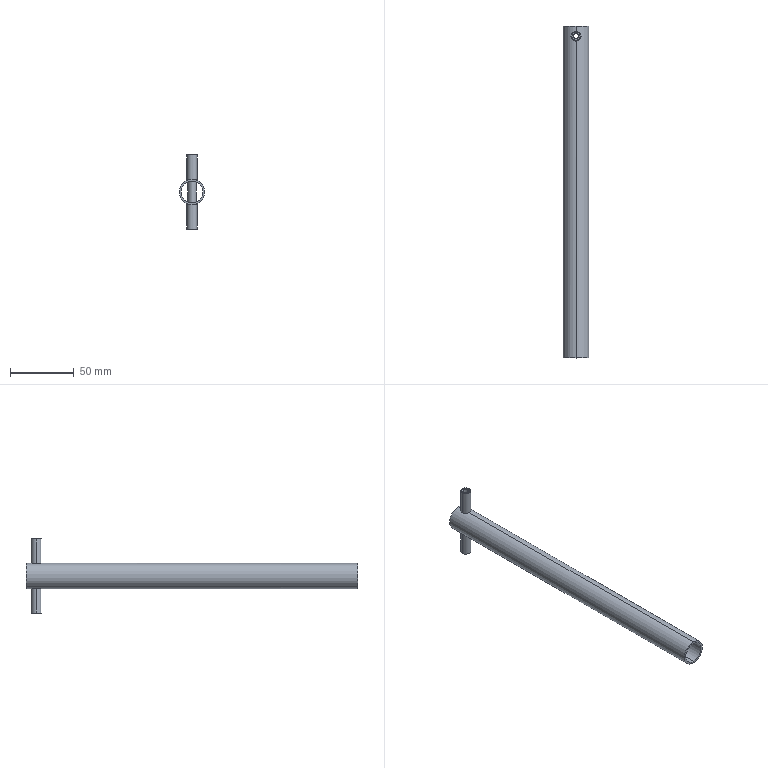Part | SolidWorks | features BaseBody 4 | 4 solids | 28 faces | box 20 x 260 x 58 mm | volume 24314 mm3 | cylinder 20 | plane 8 | commonest cylinder face diameters 6.3 x8 7.938 x4 4.166 x2 6.35 x2 17 x2 20 x2
STEP:
#1=CARTESIAN_POINT('',(0.,248.85,-10.));
#2=VERTEX_POINT('',#1);
#3=CARTESIAN_POINT('',(-3.15,252.,-9.491));
#4=VERTEX_POINT('',#3);
#5=CARTESIAN_POINT('',(0.,248.85,-10.));
#6=CARTESIAN_POINT('',(-0.2094,248.85,-10.));
#7=CARTESIAN_POINT('',(-0.4151,248.871,-9.993));
#8=CARTESIAN_POINT('',(-0.8193,248.951,-9.968));
#9=CARTESIAN_POINT('',(-1.02,249.013,-9.95));
#10=CARTESIAN_POINT('',(-1.401,249.171,-9.903));
#11=CARTESIAN_POINT('',(-1.581,249.268,-9.876));
#12=CARTESIAN_POINT('',(-1.922,249.496,-9.815));
#13=CARTESIAN_POINT('',(-2.083,249.628,-9.782));
#14=CARTESIAN_POINT('',(-2.516,250.061,-9.683));
#15=CARTESIAN_POINT('',(-2.75,250.41,-9.616));
#16=CARTESIAN_POINT('',(-2.986,250.977,-9.544));
#17=CARTESIAN_POINT('',(-3.047,251.176,-9.524));
#18=CARTESIAN_POINT('',(-3.129,251.584,-9.498));
#19=CARTESIAN_POINT('',(-3.15,251.791,-9.491));
#20=CARTESIAN_POINT('',(-3.15,252.,-9.491));
#21=B_SPLINE_CURVE_WITH_KNOTS('',3,(#5,#6,#7,#8,#9,#10,#11,#12,#13,#14,#15,#16,#17,#18,#19,#20),.UNSPECIFIED.,.F.,.F.,(4,2,2,2,2,2,2,4),(0.,0.0006191,0.001238,0.001857,0.002476,0.003715,0.004334,0.004953),.UNSPECIFIED.);
#22=EDGE_CURVE('',#2,#4,#21,.T.);
#23=ORIENTED_EDGE('',*,*,#22,.T.);
#24=CARTESIAN_POINT('',(-3.15,252.,-7.895));
#25=VERTEX_POINT('',#24);
#26=CARTESIAN_POINT('',(-3.15,252.,-10.013));
#27=DIRECTION('',(0.,0.,1.));
#28=VECTOR('',#27,1000.);
#29=LINE('',#26,#28);
#30=EDGE_CURVE('',#4,#25,#29,.T.);
#31=ORIENTED_EDGE('',*,*,#30,.T.);
#32=CARTESIAN_POINT('',(0.,248.85,-8.5));
#33=VERTEX_POINT('',#32);
#34=CARTESIAN_POINT('',(-3.15,252.,-7.895));
#35=CARTESIAN_POINT('',(-3.15,251.79,-7.895));
#36=CARTESIAN_POINT('',(-3.129,251.584,-7.903));
#37=CARTESIAN_POINT('',(-3.048,251.179,-7.935));
#38=CARTESIAN_POINT('',(-2.987,250.978,-7.958));
#39=CARTESIAN_POINT('',(-2.828,250.598,-8.016));
#40=CARTESIAN_POINT('',(-2.732,250.418,-8.05));
#41=CARTESIAN_POINT('',(-2.503,250.077,-8.124));
#42=CARTESIAN_POINT('',(-2.372,249.917,-8.164));
#43=CARTESIAN_POINT('',(-1.941,249.486,-8.281));
#44=CARTESIAN_POINT('',(-1.593,249.252,-8.358));
#45=CARTESIAN_POINT('',(-1.025,249.015,-8.44));
#46=CARTESIAN_POINT('',(-0.8254,248.953,-8.462));
#47=CARTESIAN_POINT('',(-0.4171,248.871,-8.492));
#48=CARTESIAN_POINT('',(-0.21,248.85,-8.5));
#49=CARTESIAN_POINT('',(0.,248.85,-8.5));
#50=B_SPLINE_CURVE_WITH_KNOTS('',3,(#34,#35,#36,#37,#38,#39,#40,#41,#42,#43,#44,#45,#46,#47,#48,#49),.UNSPECIFIED.,.F.,.F.,(4,2,2,2,2,2,2,4),(0.,0.0006207,0.001241,0.001862,0.002483,0.003724,0.004345,0.004966),.UNSPECIFIED.);
#51=EDGE_CURVE('',#25,#33,#50,.T.);
#52=ORIENTED_EDGE('',*,*,#51,.T.);
#53=CARTESIAN_POINT('',(3.15,252.,-7.895));
#54=VERTEX_POINT('',#53);
#55=CARTESIAN_POINT('',(0.,248.85,-8.5));
#56=CARTESIAN_POINT('',(0.21,248.85,-8.5));
#57=CARTESIAN_POINT('',(0.4162,248.871,-8.492));
#58=CARTESIAN_POINT('',(0.8212,248.952,-8.463));
#59=CARTESIAN_POINT('',(1.022,249.013,-8.441));
#60=CARTESIAN_POINT('',(1.403,249.172,-8.386));
#61=CARTESIAN_POINT('',(1.583,249.269,-8.353));
#62=CARTESIAN_POINT('',(1.924,249.497,-8.281));
#63=CARTESIAN_POINT('',(2.084,249.629,-8.242));
#64=CARTESIAN_POINT('',(2.515,250.06,-8.125));
#65=CARTESIAN_POINT('',(2.749,250.408,-8.045));
#66=CARTESIAN_POINT('',(2.986,250.975,-7.959));
#67=CARTESIAN_POINT('',(3.047,251.175,-7.935));
#68=CARTESIAN_POINT('',(3.129,251.583,-7.903));
#69=CARTESIAN_POINT('',(3.15,251.79,-7.895));
#70=CARTESIAN_POINT('',(3.15,252.,-7.895));
#71=B_SPLINE_CURVE_WITH_KNOTS('',3,(#55,#56,#57,#58,#59,#60,#61,#62,#63,#64,#65,#66,#67,#68,#69,#70),.UNSPECIFIED.,.F.,.F.,(4,2,2,2,2,2,2,4),(0.004966,0.005586,0.006207,0.006828,0.007448,0.00869,0.00931,0.009931),.UNSPECIFIED.);
#72=EDGE_CURVE('',#33,#54,#71,.T.);
#73=ORIENTED_EDGE('',*,*,#72,.T.);
#74=CARTESIAN_POINT('',(3.15,252.,-9.491));
#75=VERTEX_POINT('',#74);
#76=CARTESIAN_POINT('',(3.15,252.,-10.013));
#77=DIRECTION('',(0.,0.,1.));
#78=VECTOR('',#77,1000.);
#79=LINE('',#76,#78);
#80=EDGE_CURVE('',#75,#54,#79,.T.);
#81=ORIENTED_EDGE('',*,*,#80,.F.);
#82=CARTESIAN_POINT('',(3.15,252.,-9.491));
#83=CARTESIAN_POINT('',(3.15,251.791,-9.491));
#84=CARTESIAN_POINT('',(3.129,251.585,-9.498));
#85=CARTESIAN_POINT('',(3.049,251.181,-9.524));
#86=CARTESIAN_POINT('',(2.987,250.98,-9.544));
#87=CARTESIAN_POINT('',(2.829,250.6,-9.592));
#88=CARTESIAN_POINT('',(2.732,250.419,-9.62));
#89=CARTESIAN_POINT('',(2.504,250.078,-9.682));
#90=CARTESIAN_POINT('',(2.372,249.918,-9.716));
#91=CARTESIAN_POINT('',(1.94,249.485,-9.815));
#92=CARTESIAN_POINT('',(1.591,249.251,-9.88));
#93=CARTESIAN_POINT('',(1.024,249.014,-9.949));
#94=CARTESIAN_POINT('',(0.824,248.953,-9.968));
#95=CARTESIAN_POINT('',(0.4161,248.871,-9.993));
#96=CARTESIAN_POINT('',(0.2094,248.85,-10.));
#97=CARTESIAN_POINT('',(0.,248.85,-10.));
#98=B_SPLINE_CURVE_WITH_KNOTS('',3,(#82,#83,#84,#85,#86,#87,#88,#89,#90,#91,#92,#93,#94,#95,#96,#97),.UNSPECIFIED.,.F.,.F.,(4,2,2,2,2,2,2,4),(0.01486,0.01548,0.0161,0.01672,0.01733,0.01857,0.01919,0.01981),.UNSPECIFIED.);
#99=EDGE_CURVE('',#75,#2,#98,.T.);
#100=ORIENTED_EDGE('',*,*,#99,.T.);
#101=EDGE_LOOP('',(#23,#31,#52,#73,#81,#100));
#102=FACE_OUTER_BOUND('',#101,.T.);
#103=CARTESIAN_POINT('',(0.,252.,-10.013));
#104=DIRECTION('',(0.,0.,1.));
#105=DIRECTION('',(1.,0.,0.));
#106=AXIS2_PLACEMENT_3D('',#103,#104,#105);
#107=CYLINDRICAL_SURFACE('',#106,3.15);
#108=ADVANCED_FACE('',(#102),#107,.F.);
#109=CARTESIAN_POINT('',(0.,260.,10.));
#110=VERTEX_POINT('',#109);
#111=CARTESIAN_POINT('',(0.,260.,-10.));
#112=VERTEX_POINT('',#111);
#113=CARTESIAN_POINT('',(0.,260.,0.));
#114=DIRECTION('',(0.,1.,0.));
#115=DIRECTION('',(0.,0.,-1.));
#116=AXIS2_PLACEMENT_3D('',#113,#114,#115);
#117=CIRCLE('',#116,10.);
#118=EDGE_CURVE('',#110,#112,#117,.T.);
#119=ORIENTED_EDGE('',*,*,#118,.F.);
#120=CARTESIAN_POINT('',(0.,255.15,10.));
#121=VERTEX_POINT('',#120);
#122=CARTESIAN_POINT('',(0.,260.,10.));
#123=DIRECTION('',(0.,-1.,0.));
#124=VECTOR('',#123,1000.);
#125=LINE('',#122,#124);
#126=EDGE_CURVE('',#110,#121,#125,.T.);
#127=ORIENTED_EDGE('',*,*,#126,.T.);
#128=CARTESIAN_POINT('',(3.15,252.,9.491));
#129=VERTEX_POINT('',#128);
#130=CARTESIAN_POINT('',(3.15,252.,9.491));
#131=CARTESIAN_POINT('',(3.15,252.209,9.491));
#132=CARTESIAN_POINT('',(3.129,252.415,9.498));
#133=CARTESIAN_POINT('',(3.049,252.819,9.524));
#134=CARTESIAN_POINT('',(2.987,253.02,9.544));
#135=CARTESIAN_POINT('',(2.829,253.4,9.592));
#136=CARTESIAN_POINT('',(2.732,253.581,9.62));
#137=CARTESIAN_POINT('',(2.504,253.922,9.682));
#138=CARTESIAN_POINT('',(2.372,254.082,9.716));
#139=CARTESIAN_POINT('',(1.94,254.515,9.815));
#140=CARTESIAN_POINT('',(1.591,254.749,9.88));
#141=CARTESIAN_POINT('',(1.024,254.986,9.949));
#142=CARTESIAN_POINT('',(0.824,255.047,9.968));
#143=CARTESIAN_POINT('',(0.4161,255.129,9.993));
#144=CARTESIAN_POINT('',(0.2094,255.15,10.));
#145=CARTESIAN_POINT('',(0.,255.15,10.));
#146=B_SPLINE_CURVE_WITH_KNOTS('',3,(#130,#131,#132,#133,#134,#135,#136,#137,#138,#139,#140,#141,#142,#143,#144,#145),.UNSPECIFIED.,.F.,.F.,(4,2,2,2,2,2,2,4),(0.,0.0006191,0.001238,0.001857,0.002476,0.003714,0.004333,0.004953),.UNSPECIFIED.);
#147=EDGE_CURVE('',#129,#121,#146,.T.);
#148=ORIENTED_EDGE('',*,*,#147,.F.);
#149=CARTESIAN_POINT('',(0.,248.85,10.));
#150=VERTEX_POINT('',#149);
#151=CARTESIAN_POINT('',(0.,248.85,10.));
#152=CARTESIAN_POINT('',(0.2094,248.85,10.));
#153=CARTESIAN_POINT('',(0.4151,248.871,9.993));
#154=CARTESIAN_POINT('',(0.8193,248.951,9.968));
#155=CARTESIAN_POINT('',(1.02,249.013,9.95));
#156=CARTESIAN_POINT('',(1.401,249.171,9.903));
#157=CARTESIAN_POINT('',(1.581,249.268,9.876));
#158=CARTESIAN_POINT('',(1.922,249.496,9.815));
#159=CARTESIAN_POINT('',(2.083,249.628,9.782));
#160=CARTESIAN_POINT('',(2.516,250.061,9.683));
#161=CARTESIAN_POINT('',(2.75,250.41,9.616));
#162=CARTESIAN_POINT('',(2.986,250.977,9.544));
#163=CARTESIAN_POINT('',(3.047,251.176,9.524));
#164=CARTESIAN_POINT('',(3.129,251.584,9.498));
#165=CARTESIAN_POINT('',(3.15,251.791,9.491));
#166=CARTESIAN_POINT('',(3.15,252.,9.491));
#167=B_SPLINE_CURVE_WITH_KNOTS('',3,(#151,#152,#153,#154,#155,#156,#157,#158,#159,#160,#161,#162,#163,#164,#165,#166),.UNSPECIFIED.,.F.,.F.,(4,2,2,2,2,2,2,4),(-0.004952,-0.004333,-0.003714,-0.003095,-0.002476,-0.001238,-0.0006191,0.),.UNSPECIFIED.);
#168=EDGE_CURVE('',#150,#129,#167,.T.);
#169=ORIENTED_EDGE('',*,*,#168,.F.);
#170=CARTESIAN_POINT('',(0.,0.,10.));
#171=VERTEX_POINT('',#170);
#172=CARTESIAN_POINT('',(0.,260.,10.));
#173=DIRECTION('',(0.,-1.,0.));
#174=VECTOR('',#173,1000.);
#175=LINE('',#172,#174);
#176=EDGE_CURVE('',#150,#171,#175,.T.);
#177=ORIENTED_EDGE('',*,*,#176,.T.);
#178=CARTESIAN_POINT('',(0.,0.,-10.));
#179=VERTEX_POINT('',#178);
#180=CARTESIAN_POINT('',(0.,0.,0.));
#181=DIRECTION('',(0.,-1.,0.));
#182=DIRECTION('',(0.,0.,-1.));
#183=AXIS2_PLACEMENT_3D('',#180,#181,#182);
#184=CIRCLE('',#183,10.);
#185=EDGE_CURVE('',#179,#171,#184,.T.);
#186=ORIENTED_EDGE('',*,*,#185,.F.);
#187=CARTESIAN_POINT('',(0.,260.,-10.));
#188=DIRECTION('',(0.,-1.,0.));
#189=VECTOR('',#188,1000.);
#190=LINE('',#187,#189);
#191=EDGE_CURVE('',#2,#179,#190,.T.);
#192=ORIENTED_EDGE('',*,*,#191,.F.);
#193=ORIENTED_EDGE('',*,*,#99,.F.);
#194=CARTESIAN_POINT('',(0.,255.15,-10.));
#195=VERTEX_POINT('',#194);
#196=CARTESIAN_POINT('',(0.,255.15,-10.));
#197=CARTESIAN_POINT('',(0.2094,255.15,-10.));
#198=CARTESIAN_POINT('',(0.4151,255.129,-9.993));
#199=CARTESIAN_POINT('',(0.8193,255.049,-9.968));
#200=CARTESIAN_POINT('',(1.02,254.987,-9.95));
#201=CARTESIAN_POINT('',(1.401,254.829,-9.903));
#202=CARTESIAN_POINT('',(1.581,254.732,-9.876));
#203=CARTESIAN_POINT('',(1.922,254.504,-9.815));
#204=CARTESIAN_POINT('',(2.083,254.372,-9.782));
#205=CARTESIAN_POINT('',(2.516,253.939,-9.683));
#206=CARTESIAN_POINT('',(2.75,253.59,-9.616));
#207=CARTESIAN_POINT('',(2.986,253.023,-9.544));
#208=CARTESIAN_POINT('',(3.047,252.824,-9.524));
#209=CARTESIAN_POINT('',(3.129,252.416,-9.498));
#210=CARTESIAN_POINT('',(3.15,252.209,-9.491));
#211=CARTESIAN_POINT('',(3.15,252.,-9.491));
#212=B_SPLINE_CURVE_WITH_KNOTS('',3,(#196,#197,#198,#199,#200,#201,#202,#203,#204,#205,#206,#207,#208,#209,#210,#211),.UNSPECIFIED.,.F.,.F.,(4,2,2,2,2,2,2,4),(0.009906,0.01052,0.01114,0.01176,0.01238,0.01362,0.01424,0.01486),.UNSPECIFIED.);
#213=EDGE_CURVE('',#195,#75,#212,.T.);
#214=ORIENTED_EDGE('',*,*,#213,.F.);
#215=CARTESIAN_POINT('',(0.,260.,-10.));
#216=DIRECTION('',(0.,-1.,0.));
#217=VECTOR('',#216,1000.);
#218=LINE('',#215,#217);
#219=EDGE_CURVE('',#112,#195,#218,.T.);
#220=ORIENTED_EDGE('',*,*,#219,.F.);
#221=EDGE_LOOP('',(#119,#127,#148,#169,#177,#186,#192,#193,#214,#220));
#222=FACE_OUTER_BOUND('',#221,.T.);
#223=CARTESIAN_POINT('',(0.,260.,0.));
#224=DIRECTION('',(0.,-1.,0.));
#225=DIRECTION('',(0.,0.,-1.));
#226=AXIS2_PLACEMENT_3D('',#223,#224,#225);
#227=CYLINDRICAL_SURFACE('',#226,10.);
#228=ADVANCED_FACE('',(#222),#227,.T.);
#229=CARTESIAN_POINT('',(0.,260.,-8.5));
#230=VERTEX_POINT('',#229);
#231=CARTESIAN_POINT('',(0.,260.,8.5));
#232=VERTEX_POINT('',#231);
#233=CARTESIAN_POINT('',(0.,260.,0.));
#234=DIRECTION('',(0.,1.,0.));
#235=DIRECTION('',(0.,0.,-1.));
#236=AXIS2_PLACEMENT_3D('',#233,#234,#235);
#237=CIRCLE('',#236,8.5);
#238=EDGE_CURVE('',#230,#232,#237,.T.);
#239=ORIENTED_EDGE('',*,*,#238,.T.);
#240=CARTESIAN_POINT('',(0.,255.15,8.5));
#241=VERTEX_POINT('',#240);
#242=CARTESIAN_POINT('',(0.,260.,8.5));
#243=DIRECTION('',(0.,-1.,0.));
#244=VECTOR('',#243,1000.);
#245=LINE('',#242,#244);
#246=EDGE_CURVE('',#232,#241,#245,.T.);
#247=ORIENTED_EDGE('',*,*,#246,.T.);
#248=CARTESIAN_POINT('',(-3.15,252.,7.895));
#249=VERTEX_POINT('',#248);
#250=CARTESIAN_POINT('',(0.,255.15,8.5));
#251=CARTESIAN_POINT('',(-0.21,255.15,8.5));
#252=CARTESIAN_POINT('',(-0.4162,255.129,8.492));
#253=CARTESIAN_POINT('',(-0.8212,255.048,8.463));
#254=CARTESIAN_POINT('',(-1.022,254.987,8.441));
#255=CARTESIAN_POINT('',(-1.403,254.828,8.386));
#256=CARTESIAN_POINT('',(-1.583,254.731,8.353));
#257=CARTESIAN_POINT('',(-1.924,254.503,8.281));
#258=CARTESIAN_POINT('',(-2.084,254.371,8.242));
#259=CARTESIAN_POINT('',(-2.515,253.94,8.125));
#260=CARTESIAN_POINT('',(-2.749,253.592,8.045));
#261=CARTESIAN_POINT('',(-2.986,253.025,7.959));
#262=CARTESIAN_POINT('',(-3.047,252.825,7.935));
#263=CARTESIAN_POINT('',(-3.129,252.417,7.903));
#264=CARTESIAN_POINT('',(-3.15,252.21,7.895));
#265=CARTESIAN_POINT('',(-3.15,252.,7.895));
#266=B_SPLINE_CURVE_WITH_KNOTS('',3,(#250,#251,#252,#253,#254,#255,#256,#257,#258,#259,#260,#261,#262,#263,#264,#265),.UNSPECIFIED.,.F.,.F.,(4,2,2,2,2,2,2,4),(0.004966,0.005586,0.006207,0.006828,0.007448,0.00869,0.00931,0.009931),.UNSPECIFIED.);
#267=EDGE_CURVE('',#241,#249,#266,.T.);
#268=ORIENTED_EDGE('',*,*,#267,.T.);
#269=CARTESIAN_POINT('',(0.,248.85,8.5));
#270=VERTEX_POINT('',#269);
#271=CARTESIAN_POINT('',(-3.15,252.,7.895));
#272=CARTESIAN_POINT('',(-3.15,251.79,7.895));
#273=CARTESIAN_POINT('',(-3.129,251.584,7.903));
#274=CARTESIAN_POINT('',(-3.048,251.179,7.935));
#275=CARTESIAN_POINT('',(-2.987,250.978,7.958));
#276=CARTESIAN_POINT('',(-2.828,250.598,8.016));
#277=CARTESIAN_POINT('',(-2.732,250.418,8.05));
#278=CARTESIAN_POINT('',(-2.503,250.077,8.124));
#279=CARTESIAN_POINT('',(-2.372,249.917,8.164));
#280=CARTESIAN_POINT('',(-1.941,249.486,8.281));
#281=CARTESIAN_POINT('',(-1.593,249.252,8.358));
#282=CARTESIAN_POINT('',(-1.025,249.015,8.44));
#283=CARTESIAN_POINT('',(-0.8254,248.953,8.462));
#284=CARTESIAN_POINT('',(-0.4171,248.871,8.492));
#285=CARTESIAN_POINT('',(-0.21,248.85,8.5));
#286=CARTESIAN_POINT('',(0.,248.85,8.5));
#287=B_SPLINE_CURVE_WITH_KNOTS('',3,(#271,#272,#273,#274,#275,#276,#277,#278,#279,#280,#281,#282,#283,#284,#285,#286),.UNSPECIFIED.,.F.,.F.,(4,2,2,2,2,2,2,4),(-0.009931,-0.00931,-0.00869,-0.008069,-0.007448,-0.006207,-0.005586,-0.004966),.UNSPECIFIED.);
#288=EDGE_CURVE('',#249,#270,#287,.T.);
#289=ORIENTED_EDGE('',*,*,#288,.T.);
#290=CARTESIAN_POINT('',(0.,0.,8.5));
#291=VERTEX_POINT('',#290);
#292=CARTESIAN_POINT('',(0.,260.,8.5));
#293=DIRECTION('',(0.,-1.,0.));
#294=VECTOR('',#293,1000.);
#295=LINE('',#292,#294);
#296=EDGE_CURVE('',#270,#291,#295,.T.);
#297=ORIENTED_EDGE('',*,*,#296,.T.);
#298=CARTESIAN_POINT('',(0.,0.,-8.5));
#299=VERTEX_POINT('',#298);
#300=CARTESIAN_POINT('',(0.,0.,0.));
#301=DIRECTION('',(0.,-1.,0.));
#302=DIRECTION('',(0.,0.,-1.));
#303=AXIS2_PLACEMENT_3D('',#300,#301,#302);
#304=CIRCLE('',#303,8.5);
#305=EDGE_CURVE('',#291,#299,#304,.T.);
#306=ORIENTED_EDGE('',*,*,#305,.T.);
#307=CARTESIAN_POINT('',(0.,260.,-8.5));
#308=DIRECTION('',(0.,-1.,0.));
#309=VECTOR('',#308,1000.);
#310=LINE('',#307,#309);
#311=EDGE_CURVE('',#33,#299,#310,.T.);
#312=ORIENTED_EDGE('',*,*,#311,.F.);
#313=ORIENTED_EDGE('',*,*,#51,.F.);
#314=CARTESIAN_POINT('',(0.,255.15,-8.5));
#315=VERTEX_POINT('',#314);
#316=CARTESIAN_POINT('',(0.,255.15,-8.5));
#317=CARTESIAN_POINT('',(-0.21,255.15,-8.5));
#318=CARTESIAN_POINT('',(-0.4162,255.129,-8.492));
#319=CARTESIAN_POINT('',(-0.8212,255.048,-8.463));
#320=CARTESIAN_POINT('',(-1.022,254.987,-8.441));
#321=CARTESIAN_POINT('',(-1.403,254.828,-8.386));
#322=CARTESIAN_POINT('',(-1.583,254.731,-8.353));
#323=CARTESIAN_POINT('',(-1.924,254.503,-8.281));
#324=CARTESIAN_POINT('',(-2.084,254.371,-8.242));
#325=CARTESIAN_POINT('',(-2.515,253.94,-8.125));
#326=CARTESIAN_POINT('',(-2.749,253.592,-8.045));
#327=CARTESIAN_POINT('',(-2.986,253.025,-7.959));
#328=CARTESIAN_POINT('',(-3.047,252.825,-7.935));
#329=CARTESIAN_POINT('',(-3.129,252.417,-7.903));
#330=CARTESIAN_POINT('',(-3.15,252.21,-7.895));
#331=CARTESIAN_POINT('',(-3.15,252.,-7.895));
#332=B_SPLINE_CURVE_WITH_KNOTS('',3,(#316,#317,#318,#319,#320,#321,#322,#323,#324,#325,#326,#327,#328,#329,#330,#331),.UNSPECIFIED.,.F.,.F.,(4,2,2,2,2,2,2,4),(0.0149,0.01552,0.01614,0.01676,0.01738,0.01862,0.01924,0.01986),.UNSPECIFIED.);
#333=EDGE_CURVE('',#315,#25,#332,.T.);
#334=ORIENTED_EDGE('',*,*,#333,.F.);
#335=CARTESIAN_POINT('',(0.,260.,-8.5));
#336=DIRECTION('',(0.,-1.,0.));
#337=VECTOR('',#336,1000.);
#338=LINE('',#335,#337);
#339=EDGE_CURVE('',#230,#315,#338,.T.);
#340=ORIENTED_EDGE('',*,*,#339,.F.);
#341=EDGE_LOOP('',(#239,#247,#268,#289,#297,#306,#312,#313,#334,#340));
#342=FACE_OUTER_BOUND('',#341,.T.);
#343=CARTESIAN_POINT('',(0.,260.,0.));
#344=DIRECTION('',(0.,-1.,0.));
#345=DIRECTION('',(0.,0.,-1.));
#346=AXIS2_PLACEMENT_3D('',#343,#344,#345);
#347=CYLINDRICAL_SURFACE('',#346,8.5);
#348=ADVANCED_FACE('',(#342),#347,.F.);
#349=ORIENTED_EDGE('',*,*,#288,.F.);
#350=CARTESIAN_POINT('',(-3.15,252.,9.491));
#351=VERTEX_POINT('',#350);
#352=CARTESIAN_POINT('',(-3.15,252.,7.882));
#353=DIRECTION('',(0.,0.,1.));
#354=VECTOR('',#353,1000.);
#355=LINE('',#352,#354);
#356=EDGE_CURVE('',#249,#351,#355,.T.);
#357=ORIENTED_EDGE('',*,*,#356,.T.);
#358=CARTESIAN_POINT('',(-3.15,252.,9.491));
#359=CARTESIAN_POINT('',(-3.15,251.791,9.491));
#360=CARTESIAN_POINT('',(-3.129,251.585,9.498));
#361=CARTESIAN_POINT('',(-3.049,251.181,9.524));
#362=CARTESIAN_POINT('',(-2.987,250.98,9.544));
#363=CARTESIAN_POINT('',(-2.829,250.6,9.592));
#364=CARTESIAN_POINT('',(-2.732,250.419,9.62));
#365=CARTESIAN_POINT('',(-2.504,250.078,9.682));
#366=CARTESIAN_POINT('',(-2.372,249.918,9.716));
#367=CARTESIAN_POINT('',(-1.94,249.485,9.815));
#368=CARTESIAN_POINT('',(-1.591,249.251,9.88));
#369=CARTESIAN_POINT('',(-1.024,249.014,9.949));
#370=CARTESIAN_POINT('',(-0.824,248.953,9.968));
#371=CARTESIAN_POINT('',(-0.4161,248.871,9.993));
#372=CARTESIAN_POINT('',(-0.2094,248.85,10.));
#373=CARTESIAN_POINT('',(0.,248.85,10.));
#374=B_SPLINE_CURVE_WITH_KNOTS('',3,(#358,#359,#360,#361,#362,#363,#364,#365,#366,#367,#368,#369,#370,#371,#372,#373),.UNSPECIFIED.,.F.,.F.,(4,2,2,2,2,2,2,4),(0.009905,0.01052,0.01114,0.01176,0.01238,0.01362,0.01424,0.01486),.UNSPECIFIED.);
#375=EDGE_CURVE('',#351,#150,#374,.T.);
#376=ORIENTED_EDGE('',*,*,#375,.T.);
#377=ORIENTED_EDGE('',*,*,#168,.T.);
#378=CARTESIAN_POINT('',(3.15,252.,7.895));
#379=VERTEX_POINT('',#378);
#380=CARTESIAN_POINT('',(3.15,252.,7.882));
#381=DIRECTION('',(0.,0.,1.));
#382=VECTOR('',#381,1000.);
#383=LINE('',#380,#382);
#384=EDGE_CURVE('',#379,#129,#383,.T.);
#385=ORIENTED_EDGE('',*,*,#384,.F.);
#386=CARTESIAN_POINT('',(0.,248.85,8.5));
#387=CARTESIAN_POINT('',(0.21,248.85,8.5));
#388=CARTESIAN_POINT('',(0.4162,248.871,8.492));
#389=CARTESIAN_POINT('',(0.8212,248.952,8.463));
#390=CARTESIAN_POINT('',(1.022,249.013,8.441));
#391=CARTESIAN_POINT('',(1.403,249.172,8.386));
#392=CARTESIAN_POINT('',(1.583,249.269,8.353));
#393=CARTESIAN_POINT('',(1.924,249.497,8.281));
#394=CARTESIAN_POINT('',(2.084,249.629,8.242));
#395=CARTESIAN_POINT('',(2.515,250.06,8.125));
#396=CARTESIAN_POINT('',(2.749,250.408,8.045));
#397=CARTESIAN_POINT('',(2.986,250.975,7.959));
#398=CARTESIAN_POINT('',(3.047,251.175,7.935));
#399=CARTESIAN_POINT('',(3.129,251.583,7.903));
#400=CARTESIAN_POINT('',(3.15,251.79,7.895));
#401=CARTESIAN_POINT('',(3.15,252.,7.895));
#402=B_SPLINE_CURVE_WITH_KNOTS('',3,(#386,#387,#388,#389,#390,#391,#392,#393,#394,#395,#396,#397,#398,#399,#400,#401),.UNSPECIFIED.,.F.,.F.,(4,2,2,2,2,2,2,4),(-0.004966,-0.004345,-0.003724,-0.003103,-0.002483,-0.001241,-0.0006207,0.),.UNSPECIFIED.);
#403=EDGE_CURVE('',#270,#379,#402,.T.);
#404=ORIENTED_EDGE('',*,*,#403,.F.);
#405=EDGE_LOOP('',(#349,#357,#376,#377,#385,#404));
#406=FACE_OUTER_BOUND('',#405,.T.);
#407=CARTESIAN_POINT('',(0.,252.,7.882));
#408=DIRECTION('',(0.,0.,1.));
#409=DIRECTION('',(1.,0.,0.));
#410=AXIS2_PLACEMENT_3D('',#407,#408,#409);
#411=CYLINDRICAL_SURFACE('',#410,3.15);
#412=ADVANCED_FACE('',(#406),#411,.F.);
#413=ORIENTED_EDGE('',*,*,#30,.F.);
#414=CARTESIAN_POINT('',(-3.15,252.,-9.491));
#415=CARTESIAN_POINT('',(-3.15,252.209,-9.491));
#416=CARTESIAN_POINT('',(-3.129,252.415,-9.498));
#417=CARTESIAN_POINT('',(-3.049,252.819,-9.524));
#418=CARTESIAN_POINT('',(-2.987,253.02,-9.544));
#419=CARTESIAN_POINT('',(-2.829,253.4,-9.592));
#420=CARTESIAN_POINT('',(-2.732,253.581,-9.62));
#421=CARTESIAN_POINT('',(-2.504,253.922,-9.682));
#422=CARTESIAN_POINT('',(-2.372,254.082,-9.716));
#423=CARTESIAN_POINT('',(-1.94,254.515,-9.815));
#424=CARTESIAN_POINT('',(-1.591,254.749,-9.88));
#425=CARTESIAN_POINT('',(-1.024,254.986,-9.949));
#426=CARTESIAN_POINT('',(-0.824,255.047,-9.968));
#427=CARTESIAN_POINT('',(-0.4161,255.129,-9.993));
#428=CARTESIAN_POINT('',(-0.2094,255.15,-10.));
#429=CARTESIAN_POINT('',(0.,255.15,-10.));
#430=B_SPLINE_CURVE_WITH_KNOTS('',3,(#414,#415,#416,#417,#418,#419,#420,#421,#422,#423,#424,#425,#426,#427,#428,#429),.UNSPECIFIED.,.F.,.F.,(4,2,2,2,2,2,2,4),(0.004953,0.005572,0.006191,0.00681,0.007429,0.008667,0.009286,0.009906),.UNSPECIFIED.);
#431=EDGE_CURVE('',#4,#195,#430,.T.);
#432=ORIENTED_EDGE('',*,*,#431,.T.);
#433=ORIENTED_EDGE('',*,*,#213,.T.);
#434=ORIENTED_EDGE('',*,*,#80,.T.);
#435=CARTESIAN_POINT('',(3.15,252.,-7.895));
#436=CARTESIAN_POINT('',(3.15,252.21,-7.895));
#437=CARTESIAN_POINT('',(3.129,252.416,-7.903));
#438=CARTESIAN_POINT('',(3.048,252.821,-7.935));
#439=CARTESIAN_POINT('',(2.987,253.022,-7.958));
#440=CARTESIAN_POINT('',(2.828,253.402,-8.016));
#441=CARTESIAN_POINT('',(2.732,253.582,-8.05));
#442=CARTESIAN_POINT('',(2.503,253.923,-8.124));
#443=CARTESIAN_POINT('',(2.372,254.083,-8.164));
#444=CARTESIAN_POINT('',(1.941,254.514,-8.281));
#445=CARTESIAN_POINT('',(1.593,254.748,-8.358));
#446=CARTESIAN_POINT('',(1.025,254.985,-8.44));
#447=CARTESIAN_POINT('',(0.8254,255.047,-8.462));
#448=CARTESIAN_POINT('',(0.4171,255.129,-8.492));
#449=CARTESIAN_POINT('',(0.21,255.15,-8.5));
#450=CARTESIAN_POINT('',(0.,255.15,-8.5));
#451=B_SPLINE_CURVE_WITH_KNOTS('',3,(#435,#436,#437,#438,#439,#440,#441,#442,#443,#444,#445,#446,#447,#448,#449,#450),.UNSPECIFIED.,.F.,.F.,(4,2,2,2,2,2,2,4),(0.009931,0.01055,0.01117,0.01179,0.01241,0.01366,0.01428,0.0149),.UNSPECIFIED.);
#452=EDGE_CURVE('',#54,#315,#451,.T.);
#453=ORIENTED_EDGE('',*,*,#452,.T.);
#454=ORIENTED_EDGE('',*,*,#333,.T.);
#455=EDGE_LOOP('',(#413,#432,#433,#434,#453,#454));
#456=FACE_OUTER_BOUND('',#455,.T.);
#457=CARTESIAN_POINT('',(0.,252.,-10.013));
#458=DIRECTION('',(0.,0.,1.));
#459=DIRECTION('',(1.,0.,0.));
#460=AXIS2_PLACEMENT_3D('',#457,#458,#459);
#461=CYLINDRICAL_SURFACE('',#460,3.15);
#462=ADVANCED_FACE('',(#456),#461,.F.);
#463=ORIENTED_EDGE('',*,*,#126,.F.);
#464=CARTESIAN_POINT('',(0.,260.,0.));
#465=DIRECTION('',(0.,1.,0.));
#466=DIRECTION('',(0.,0.,-1.));
#467=AXIS2_PLACEMENT_3D('',#464,#465,#466);
#468=CIRCLE('',#467,10.);
#469=EDGE_CURVE('',#112,#110,#468,.T.);
#470=ORIENTED_EDGE('',*,*,#469,.F.);
#471=ORIENTED_EDGE('',*,*,#219,.T.);
#472=ORIENTED_EDGE('',*,*,#431,.F.);
#473=ORIENTED_EDGE('',*,*,#22,.F.);
#474=ORIENTED_EDGE('',*,*,#191,.T.);
#475=CARTESIAN_POINT('',(0.,0.,0.));
#476=DIRECTION('',(0.,-1.,0.));
#477=DIRECTION('',(0.,0.,-1.));
#478=AXIS2_PLACEMENT_3D('',#475,#476,#477);
#479=CIRCLE('',#478,10.);
#480=EDGE_CURVE('',#171,#179,#479,.T.);
#481=ORIENTED_EDGE('',*,*,#480,.F.);
#482=ORIENTED_EDGE('',*,*,#176,.F.);
#483=ORIENTED_EDGE('',*,*,#375,.F.);
#484=CARTESIAN_POINT('',(0.,255.15,10.));
#485=CARTESIAN_POINT('',(-0.2094,255.15,10.));
#486=CARTESIAN_POINT('',(-0.4151,255.129,9.993));
#487=CARTESIAN_POINT('',(-0.8193,255.049,9.968));
#488=CARTESIAN_POINT('',(-1.02,254.987,9.95));
#489=CARTESIAN_POINT('',(-1.401,254.829,9.903));
#490=CARTESIAN_POINT('',(-1.581,254.732,9.876));
#491=CARTESIAN_POINT('',(-1.922,254.504,9.815));
#492=CARTESIAN_POINT('',(-2.083,254.372,9.782));
#493=CARTESIAN_POINT('',(-2.516,253.939,9.683));
#494=CARTESIAN_POINT('',(-2.75,253.59,9.616));
#495=CARTESIAN_POINT('',(-2.986,253.023,9.544));
#496=CARTESIAN_POINT('',(-3.047,252.824,9.524));
#497=CARTESIAN_POINT('',(-3.129,252.416,9.498));
#498=CARTESIAN_POINT('',(-3.15,252.209,9.491));
#499=CARTESIAN_POINT('',(-3.15,252.,9.491));
#500=B_SPLINE_CURVE_WITH_KNOTS('',3,(#484,#485,#486,#487,#488,#489,#490,#491,#492,#493,#494,#495,#496,#497,#498,#499),.UNSPECIFIED.,.F.,.F.,(4,2,2,2,2,2,2,4),(0.004953,0.005572,0.006191,0.00681,0.007429,0.008667,0.009286,0.009905),.UNSPECIFIED.);
#501=EDGE_CURVE('',#121,#351,#500,.T.);
#502=ORIENTED_EDGE('',*,*,#501,.F.);
#503=EDGE_LOOP('',(#463,#470,#471,#472,#473,#474,#481,#482,#483,#502));
#504=FACE_OUTER_BOUND('',#503,.T.);
#505=CARTESIAN_POINT('',(0.,260.,0.));
#506=DIRECTION('',(0.,-1.,0.));
#507=DIRECTION('',(0.,0.,-1.));
#508=AXIS2_PLACEMENT_3D('',#505,#506,#507);
#509=CYLINDRICAL_SURFACE('',#508,10.);
#510=ADVANCED_FACE('',(#504),#509,.T.);
#511=ORIENTED_EDGE('',*,*,#246,.F.);
#512=CARTESIAN_POINT('',(0.,260.,0.));
#513=DIRECTION('',(0.,1.,0.));
#514=DIRECTION('',(0.,0.,-1.));
#515=AXIS2_PLACEMENT_3D('',#512,#513,#514);
#516=CIRCLE('',#515,8.5);
#517=EDGE_CURVE('',#232,#230,#516,.T.);
#518=ORIENTED_EDGE('',*,*,#517,.T.);
#519=ORIENTED_EDGE('',*,*,#339,.T.);
#520=ORIENTED_EDGE('',*,*,#452,.F.);
#521=ORIENTED_EDGE('',*,*,#72,.F.);
#522=ORIENTED_EDGE('',*,*,#311,.T.);
#523=CARTESIAN_POINT('',(0.,0.,0.));
#524=DIRECTION('',(0.,-1.,0.));
#525=DIRECTION('',(0.,0.,-1.));
#526=AXIS2_PLACEMENT_3D('',#523,#524,#525);
#527=CIRCLE('',#526,8.5);
#528=EDGE_CURVE('',#299,#291,#527,.T.);
#529=ORIENTED_EDGE('',*,*,#528,.T.);
#530=ORIENTED_EDGE('',*,*,#296,.F.);
#531=ORIENTED_EDGE('',*,*,#403,.T.);
#532=CARTESIAN_POINT('',(3.15,252.,7.895));
#533=CARTESIAN_POINT('',(3.15,252.21,7.895));
#534=CARTESIAN_POINT('',(3.129,252.416,7.903));
#535=CARTESIAN_POINT('',(3.048,252.821,7.935));
#536=CARTESIAN_POINT('',(2.987,253.022,7.958));
#537=CARTESIAN_POINT('',(2.828,253.402,8.016));
#538=CARTESIAN_POINT('',(2.732,253.582,8.05));
#539=CARTESIAN_POINT('',(2.503,253.923,8.124));
#540=CARTESIAN_POINT('',(2.372,254.083,8.164));
#541=CARTESIAN_POINT('',(1.941,254.514,8.281));
#542=CARTESIAN_POINT('',(1.593,254.748,8.358));
#543=CARTESIAN_POINT('',(1.025,254.985,8.44));
#544=CARTESIAN_POINT('',(0.8254,255.047,8.462));
#545=CARTESIAN_POINT('',(0.4171,255.129,8.492));
#546=CARTESIAN_POINT('',(0.21,255.15,8.5));
#547=CARTESIAN_POINT('',(0.,255.15,8.5));
#548=B_SPLINE_CURVE_WITH_KNOTS('',3,(#532,#533,#534,#535,#536,#537,#538,#539,#540,#541,#542,#543,#544,#545,#546,#547),.UNSPECIFIED.,.F.,.F.,(4,2,2,2,2,2,2,4),(0.,0.0006207,0.001241,0.001862,0.002483,0.003724,0.004345,0.004966),.UNSPECIFIED.);
#549=EDGE_CURVE('',#379,#241,#548,.T.);
#550=ORIENTED_EDGE('',*,*,#549,.T.);
#551=EDGE_LOOP('',(#511,#518,#519,#520,#521,#522,#529,#530,#531,#550));
#552=FACE_OUTER_BOUND('',#551,.T.);
#553=CARTESIAN_POINT('',(0.,260.,0.));
#554=DIRECTION('',(0.,-1.,0.));
#555=DIRECTION('',(0.,0.,-1.));
#556=AXIS2_PLACEMENT_3D('',#553,#554,#555);
#557=CYLINDRICAL_SURFACE('',#556,8.5);
#558=ADVANCED_FACE('',(#552),#557,.F.);
#559=ORIENTED_EDGE('',*,*,#238,.F.);
#560=ORIENTED_EDGE('',*,*,#517,.F.);
#561=EDGE_LOOP('',(#559,#560));
#562=FACE_BOUND('',#561,.T.);
#563=ORIENTED_EDGE('',*,*,#469,.T.);
#564=ORIENTED_EDGE('',*,*,#118,.T.);
#565=EDGE_LOOP('',(#563,#564));
#566=FACE_OUTER_BOUND('',#565,.T.);
#567=CARTESIAN_POINT('',(-10.12,260.,-10.12));
#568=DIRECTION('',(0.,1.,0.));
#569=DIRECTION('',(0.,0.,1.));
#570=AXIS2_PLACEMENT_3D('',#567,#568,#569);
#571=PLANE('',#570);
#572=ADVANCED_FACE('',(#562,#566),#571,.T.);
#573=ORIENTED_EDGE('',*,*,#356,.F.);
#574=ORIENTED_EDGE('',*,*,#267,.F.);
#575=ORIENTED_EDGE('',*,*,#549,.F.);
#576=ORIENTED_EDGE('',*,*,#384,.T.);
#577=ORIENTED_EDGE('',*,*,#147,.T.);
#578=ORIENTED_EDGE('',*,*,#501,.T.);
#579=EDGE_LOOP('',(#573,#574,#575,#576,#577,#578));
#580=FACE_OUTER_BOUND('',#579,.T.);
#581=CARTESIAN_POINT('',(0.,252.,7.882));
#582=DIRECTION('',(0.,0.,1.));
#583=DIRECTION('',(1.,0.,0.));
#584=AXIS2_PLACEMENT_3D('',#581,#582,#583);
#585=CYLINDRICAL_SURFACE('',#584,3.15);
#586=ADVANCED_FACE('',(#580),#585,.F.);
#587=ORIENTED_EDGE('',*,*,#528,.F.);
#588=ORIENTED_EDGE('',*,*,#305,.F.);
#589=EDGE_LOOP('',(#587,#588));
#590=FACE_BOUND('',#589,.T.);
#591=ORIENTED_EDGE('',*,*,#185,.T.);
#592=ORIENTED_EDGE('',*,*,#480,.T.);
#593=EDGE_LOOP('',(#591,#592));
#594=FACE_OUTER_BOUND('',#593,.T.);
#595=CARTESIAN_POINT('',(-10.12,0.,-10.12));
#596=DIRECTION('',(0.,1.,0.));
#597=DIRECTION('',(0.,0.,1.));
#598=AXIS2_PLACEMENT_3D('',#595,#596,#597);
#599=PLANE('',#598);
#600=ADVANCED_FACE('',(#590,#594),#599,.F.);
#601=CLOSED_SHELL('',(#108,#228,#348,#412,#462,#510,#558,#572,#586,#600));
#602=MANIFOLD_SOLID_BREP('',#601);
#603=CARTESIAN_POINT('',(-2.083,252.,29.));
#604=VERTEX_POINT('',#603);
#605=CARTESIAN_POINT('',(2.083,252.,29.));
#606=VERTEX_POINT('',#605);
#607=CARTESIAN_POINT('',(0.,252.,29.));
#608=DIRECTION('',(0.,0.,1.));
#609=DIRECTION('',(-1.,0.,0.));
#610=AXIS2_PLACEMENT_3D('',#607,#608,#609);
#611=CIRCLE('',#610,2.083);
#612=EDGE_CURVE('',#604,#606,#611,.T.);
#613=ORIENTED_EDGE('',*,*,#612,.T.);
#614=CARTESIAN_POINT('',(2.083,252.,-29.));
#615=VERTEX_POINT('',#614);
#616=CARTESIAN_POINT('',(2.083,252.,29.));
#617=DIRECTION('',(0.,0.,-1.));
#618=VECTOR('',#617,1000.);
#619=LINE('',#616,#618);
#620=EDGE_CURVE('',#606,#615,#619,.T.);
#621=ORIENTED_EDGE('',*,*,#620,.T.);
#622=CARTESIAN_POINT('',(-2.083,252.,-29.));
#623=VERTEX_POINT('',#622);
#624=CARTESIAN_POINT('',(0.,252.,-29.));
#625=DIRECTION('',(0.,0.,-1.));
#626=DIRECTION('',(-1.,0.,0.));
#627=AXIS2_PLACEMENT_3D('',#624,#625,#626);
#628=CIRCLE('',#627,2.083);
#629=EDGE_CURVE('',#615,#623,#628,.T.);
#630=ORIENTED_EDGE('',*,*,#629,.T.);
#631=CARTESIAN_POINT('',(-2.083,252.,29.));
#632=DIRECTION('',(0.,0.,-1.));
#633=VECTOR('',#632,1000.);
#634=LINE('',#631,#633);
#635=EDGE_CURVE('',#604,#623,#634,.T.);
#636=ORIENTED_EDGE('',*,*,#635,.F.);
#637=EDGE_LOOP('',(#613,#621,#630,#636));
#638=FACE_OUTER_BOUND('',#637,.T.);
#639=CARTESIAN_POINT('',(0.,252.,29.));
#640=DIRECTION('',(0.,0.,-1.));
#641=DIRECTION('',(-1.,0.,0.));
#642=AXIS2_PLACEMENT_3D('',#639,#640,#641);
#643=CYLINDRICAL_SURFACE('',#642,2.083);
#644=ADVANCED_FACE('',(#638),#643,.F.);
#645=CARTESIAN_POINT('',(3.175,252.,29.));
#646=VERTEX_POINT('',#645);
#647=CARTESIAN_POINT('',(-3.175,252.,29.));
#648=VERTEX_POINT('',#647);
#649=CARTESIAN_POINT('',(0.,252.,29.));
#650=DIRECTION('',(0.,0.,1.));
#651=DIRECTION('',(-1.,0.,0.));
#652=AXIS2_PLACEMENT_3D('',#649,#650,#651);
#653=CIRCLE('',#652,3.175);
#654=EDGE_CURVE('',#646,#648,#653,.T.);
#655=ORIENTED_EDGE('',*,*,#654,.F.);
#656=CARTESIAN_POINT('',(3.175,252.,-29.));
#657=VERTEX_POINT('',#656);
#658=CARTESIAN_POINT('',(3.175,252.,29.));
#659=DIRECTION('',(0.,0.,-1.));
#660=VECTOR('',#659,1000.);
#661=LINE('',#658,#660);
#662=EDGE_CURVE('',#646,#657,#661,.T.);
#663=ORIENTED_EDGE('',*,*,#662,.T.);
#664=CARTESIAN_POINT('',(-3.175,252.,-29.));
#665=VERTEX_POINT('',#664);
#666=CARTESIAN_POINT('',(0.,252.,-29.));
#667=DIRECTION('',(0.,0.,1.));
#668=DIRECTION('',(-1.,0.,0.));
#669=AXIS2_PLACEMENT_3D('',#666,#667,#668);
#670=CIRCLE('',#669,3.175);
#671=EDGE_CURVE('',#657,#665,#670,.T.);
#672=ORIENTED_EDGE('',*,*,#671,.T.);
#673=CARTESIAN_POINT('',(-3.175,252.,29.));
#674=DIRECTION('',(0.,0.,-1.));
#675=VECTOR('',#674,1000.);
#676=LINE('',#673,#675);
#677=EDGE_CURVE('',#648,#665,#676,.T.);
#678=ORIENTED_EDGE('',*,*,#677,.F.);
#679=EDGE_LOOP('',(#655,#663,#672,#678));
#680=FACE_OUTER_BOUND('',#679,.T.);
#681=CARTESIAN_POINT('',(0.,252.,29.));
#682=DIRECTION('',(0.,0.,-1.));
#683=DIRECTION('',(-1.,0.,0.));
#684=AXIS2_PLACEMENT_3D('',#681,#682,#683);
#685=CYLINDRICAL_SURFACE('',#684,3.175);
#686=ADVANCED_FACE('',(#680),#685,.T.);
#687=ORIENTED_EDGE('',*,*,#620,.F.);
#688=CARTESIAN_POINT('',(0.,252.,29.));
#689=DIRECTION('',(0.,0.,1.));
#690=DIRECTION('',(-1.,0.,0.));
#691=AXIS2_PLACEMENT_3D('',#688,#689,#690);
#692=CIRCLE('',#691,2.083);
#693=EDGE_CURVE('',#606,#604,#692,.T.);
#694=ORIENTED_EDGE('',*,*,#693,.T.);
#695=ORIENTED_EDGE('',*,*,#635,.T.);
#696=CARTESIAN_POINT('',(0.,252.,-29.));
#697=DIRECTION('',(0.,0.,-1.));
#698=DIRECTION('',(-1.,0.,0.));
#699=AXIS2_PLACEMENT_3D('',#696,#697,#698);
#700=CIRCLE('',#699,2.083);
#701=EDGE_CURVE('',#623,#615,#700,.T.);
#702=ORIENTED_EDGE('',*,*,#701,.T.);
#703=EDGE_LOOP('',(#687,#694,#695,#702));
#704=FACE_OUTER_BOUND('',#703,.T.);
#705=CARTESIAN_POINT('',(0.,252.,29.));
#706=DIRECTION('',(0.,0.,-1.));
#707=DIRECTION('',(-1.,0.,0.));
#708=AXIS2_PLACEMENT_3D('',#705,#706,#707);
#709=CYLINDRICAL_SURFACE('',#708,2.083);
#710=ADVANCED_FACE('',(#704),#709,.F.);
#711=ORIENTED_EDGE('',*,*,#701,.F.);
#712=ORIENTED_EDGE('',*,*,#629,.F.);
#713=EDGE_LOOP('',(#711,#712));
#714=FACE_BOUND('',#713,.T.);
#715=CARTESIAN_POINT('',(0.,252.,-29.));
#716=DIRECTION('',(0.,0.,1.));
#717=DIRECTION('',(-1.,0.,0.));
#718=AXIS2_PLACEMENT_3D('',#715,#716,#717);
#719=CIRCLE('',#718,3.175);
#720=EDGE_CURVE('',#665,#657,#719,.T.);
#721=ORIENTED_EDGE('',*,*,#720,.F.);
#722=ORIENTED_EDGE('',*,*,#671,.F.);
#723=EDGE_LOOP('',(#721,#722));
#724=FACE_OUTER_BOUND('',#723,.T.);
#725=CARTESIAN_POINT('',(-3.213,248.787,-29.));
#726=DIRECTION('',(0.,0.,1.));
#727=DIRECTION('',(1.,0.,0.));
#728=AXIS2_PLACEMENT_3D('',#725,#726,#727);
#729=PLANE('',#728);
#730=ADVANCED_FACE('',(#714,#724),#729,.F.);
#731=ORIENTED_EDGE('',*,*,#612,.F.);
#732=ORIENTED_EDGE('',*,*,#693,.F.);
#733=EDGE_LOOP('',(#731,#732));
#734=FACE_BOUND('',#733,.T.);
#735=CARTESIAN_POINT('',(0.,252.,29.));
#736=DIRECTION('',(0.,0.,1.));
#737=DIRECTION('',(-1.,0.,0.));
#738=AXIS2_PLACEMENT_3D('',#735,#736,#737);
#739=CIRCLE('',#738,3.175);
#740=EDGE_CURVE('',#648,#646,#739,.T.);
#741=ORIENTED_EDGE('',*,*,#740,.T.);
#742=ORIENTED_EDGE('',*,*,#654,.T.);
#743=EDGE_LOOP('',(#741,#742));
#744=FACE_OUTER_BOUND('',#743,.T.);
#745=CARTESIAN_POINT('',(-3.213,248.787,29.));
#746=DIRECTION('',(0.,0.,1.));
#747=DIRECTION('',(1.,0.,0.));
#748=AXIS2_PLACEMENT_3D('',#745,#746,#747);
#749=PLANE('',#748);
#750=ADVANCED_FACE('',(#734,#744),#749,.T.);
#751=ORIENTED_EDGE('',*,*,#662,.F.);
#752=ORIENTED_EDGE('',*,*,#740,.F.);
#753=ORIENTED_EDGE('',*,*,#677,.T.);
#754=ORIENTED_EDGE('',*,*,#720,.T.);
#755=EDGE_LOOP('',(#751,#752,#753,#754));
#756=FACE_OUTER_BOUND('',#755,.T.);
#757=CARTESIAN_POINT('',(0.,252.,29.));
#758=DIRECTION('',(0.,0.,-1.));
#759=DIRECTION('',(-1.,0.,0.));
#760=AXIS2_PLACEMENT_3D('',#757,#758,#759);
#761=CYLINDRICAL_SURFACE('',#760,3.175);
#762=ADVANCED_FACE('',(#756),#761,.T.);
#763=CLOSED_SHELL('',(#644,#686,#710,#730,#750,#762));
#764=MANIFOLD_SOLID_BREP('',#763);
#765=CARTESIAN_POINT('',(-3.15,252.,29.));
#766=VERTEX_POINT('',#765);
#767=CARTESIAN_POINT('',(3.15,252.,29.));
#768=VERTEX_POINT('',#767);
#769=CARTESIAN_POINT('',(0.,252.,29.));
#770=DIRECTION('',(0.,0.,1.));
#771=DIRECTION('',(-1.,0.,0.));
#772=AXIS2_PLACEMENT_3D('',#769,#770,#771);
#773=CIRCLE('',#772,3.15);
#774=EDGE_CURVE('',#766,#768,#773,.T.);
#775=ORIENTED_EDGE('',*,*,#774,.T.);
#776=CARTESIAN_POINT('',(3.15,252.,10.));
#777=VERTEX_POINT('',#776);
#778=CARTESIAN_POINT('',(3.15,252.,29.));
#779=DIRECTION('',(0.,0.,-1.));
#780=VECTOR('',#779,1000.);
#781=LINE('',#778,#780);
#782=EDGE_CURVE('',#768,#777,#781,.T.);
#783=ORIENTED_EDGE('',*,*,#782,.T.);
#784=CARTESIAN_POINT('',(-3.15,252.,10.));
#785=VERTEX_POINT('',#784);
#786=CARTESIAN_POINT('',(0.,252.,10.));
#787=DIRECTION('',(0.,0.,-1.));
#788=DIRECTION('',(-1.,0.,0.));
#789=AXIS2_PLACEMENT_3D('',#786,#787,#788);
#790=CIRCLE('',#789,3.15);
#791=EDGE_CURVE('',#777,#785,#790,.T.);
#792=ORIENTED_EDGE('',*,*,#791,.T.);
#793=CARTESIAN_POINT('',(-3.15,252.,29.));
#794=DIRECTION('',(0.,0.,-1.));
#795=VECTOR('',#794,1000.);
#796=LINE('',#793,#795);
#797=EDGE_CURVE('',#766,#785,#796,.T.);
#798=ORIENTED_EDGE('',*,*,#797,.F.);
#799=EDGE_LOOP('',(#775,#783,#792,#798));
#800=FACE_OUTER_BOUND('',#799,.T.);
#801=CARTESIAN_POINT('',(0.,252.,29.));
#802=DIRECTION('',(0.,0.,-1.));
#803=DIRECTION('',(-1.,0.,0.));
#804=AXIS2_PLACEMENT_3D('',#801,#802,#803);
#805=CYLINDRICAL_SURFACE('',#804,3.15);
#806=ADVANCED_FACE('',(#800),#805,.F.);
#807=CARTESIAN_POINT('',(3.969,252.,29.));
#808=VERTEX_POINT('',#807);
#809=CARTESIAN_POINT('',(-3.969,252.,29.));
#810=VERTEX_POINT('',#809);
#811=CARTESIAN_POINT('',(0.,252.,29.));
#812=DIRECTION('',(0.,0.,1.));
#813=DIRECTION('',(-1.,0.,0.));
#814=AXIS2_PLACEMENT_3D('',#811,#812,#813);
#815=CIRCLE('',#814,3.969);
#816=EDGE_CURVE('',#808,#810,#815,.T.);
#817=ORIENTED_EDGE('',*,*,#816,.F.);
#818=CARTESIAN_POINT('',(3.969,252.,10.));
#819=VERTEX_POINT('',#818);
#820=CARTESIAN_POINT('',(3.969,252.,29.));
#821=DIRECTION('',(0.,0.,-1.));
#822=VECTOR('',#821,1000.);
#823=LINE('',#820,#822);
#824=EDGE_CURVE('',#808,#819,#823,.T.);
#825=ORIENTED_EDGE('',*,*,#824,.T.);
#826=CARTESIAN_POINT('',(-3.969,252.,10.));
#827=VERTEX_POINT('',#826);
#828=CARTESIAN_POINT('',(0.,252.,10.));
#829=DIRECTION('',(0.,0.,1.));
#830=DIRECTION('',(-1.,0.,0.));
#831=AXIS2_PLACEMENT_3D('',#828,#829,#830);
#832=CIRCLE('',#831,3.969);
#833=EDGE_CURVE('',#819,#827,#832,.T.);
#834=ORIENTED_EDGE('',*,*,#833,.T.);
#835=CARTESIAN_POINT('',(-3.969,252.,29.));
#836=DIRECTION('',(0.,0.,-1.));
#837=VECTOR('',#836,1000.);
#838=LINE('',#835,#837);
#839=EDGE_CURVE('',#810,#827,#838,.T.);
#840=ORIENTED_EDGE('',*,*,#839,.F.);
#841=EDGE_LOOP('',(#817,#825,#834,#840));
#842=FACE_OUTER_BOUND('',#841,.T.);
#843=CARTESIAN_POINT('',(0.,252.,29.));
#844=DIRECTION('',(0.,0.,-1.));
#845=DIRECTION('',(-1.,0.,0.));
#846=AXIS2_PLACEMENT_3D('',#843,#844,#845);
#847=CYLINDRICAL_SURFACE('',#846,3.969);
#848=ADVANCED_FACE('',(#842),#847,.T.);
#849=ORIENTED_EDGE('',*,*,#782,.F.);
#850=CARTESIAN_POINT('',(0.,252.,29.));
#851=DIRECTION('',(0.,0.,1.));
#852=DIRECTION('',(-1.,0.,0.));
#853=AXIS2_PLACEMENT_3D('',#850,#851,#852);
#854=CIRCLE('',#853,3.15);
#855=EDGE_CURVE('',#768,#766,#854,.T.);
#856=ORIENTED_EDGE('',*,*,#855,.T.);
#857=ORIENTED_EDGE('',*,*,#797,.T.);
#858=CARTESIAN_POINT('',(0.,252.,10.));
#859=DIRECTION('',(0.,0.,-1.));
#860=DIRECTION('',(-1.,0.,0.));
#861=AXIS2_PLACEMENT_3D('',#858,#859,#860);
#862=CIRCLE('',#861,3.15);
#863=EDGE_CURVE('',#785,#777,#862,.T.);
#864=ORIENTED_EDGE('',*,*,#863,.T.);
#865=EDGE_LOOP('',(#849,#856,#857,#864));
#866=FACE_OUTER_BOUND('',#865,.T.);
#867=CARTESIAN_POINT('',(0.,252.,29.));
#868=DIRECTION('',(0.,0.,-1.));
#869=DIRECTION('',(-1.,0.,0.));
#870=AXIS2_PLACEMENT_3D('',#867,#868,#869);
#871=CYLINDRICAL_SURFACE('',#870,3.15);
#872=ADVANCED_FACE('',(#866),#871,.F.);
#873=ORIENTED_EDGE('',*,*,#863,.F.);
#874=ORIENTED_EDGE('',*,*,#791,.F.);
#875=EDGE_LOOP('',(#873,#874));
#876=FACE_BOUND('',#875,.T.);
#877=CARTESIAN_POINT('',(0.,252.,10.));
#878=DIRECTION('',(0.,0.,1.));
#879=DIRECTION('',(-1.,0.,0.));
#880=AXIS2_PLACEMENT_3D('',#877,#878,#879);
#881=CIRCLE('',#880,3.969);
#882=EDGE_CURVE('',#827,#819,#881,.T.);
#883=ORIENTED_EDGE('',*,*,#882,.F.);
#884=ORIENTED_EDGE('',*,*,#833,.F.);
#885=EDGE_LOOP('',(#883,#884));
#886=FACE_OUTER_BOUND('',#885,.T.);
#887=CARTESIAN_POINT('',(-4.016,247.984,10.));
#888=DIRECTION('',(0.,0.,1.));
#889=DIRECTION('',(1.,0.,0.));
#890=AXIS2_PLACEMENT_3D('',#887,#888,#889);
#891=PLANE('',#890);
#892=ADVANCED_FACE('',(#876,#886),#891,.F.);
#893=ORIENTED_EDGE('',*,*,#774,.F.);
#894=ORIENTED_EDGE('',*,*,#855,.F.);
#895=EDGE_LOOP('',(#893,#894));
#896=FACE_BOUND('',#895,.T.);
#897=CARTESIAN_POINT('',(0.,252.,29.));
#898=DIRECTION('',(0.,0.,1.));
#899=DIRECTION('',(-1.,0.,0.));
#900=AXIS2_PLACEMENT_3D('',#897,#898,#899);
#901=CIRCLE('',#900,3.969);
#902=EDGE_CURVE('',#810,#808,#901,.T.);
#903=ORIENTED_EDGE('',*,*,#902,.T.);
#904=ORIENTED_EDGE('',*,*,#816,.T.);
#905=EDGE_LOOP('',(#903,#904));
#906=FACE_OUTER_BOUND('',#905,.T.);
#907=CARTESIAN_POINT('',(-4.016,247.984,29.));
#908=DIRECTION('',(0.,0.,1.));
#909=DIRECTION('',(1.,0.,0.));
#910=AXIS2_PLACEMENT_3D('',#907,#908,#909);
#911=PLANE('',#910);
#912=ADVANCED_FACE('',(#896,#906),#911,.T.);
#913=ORIENTED_EDGE('',*,*,#824,.F.);
#914=ORIENTED_EDGE('',*,*,#902,.F.);
#915=ORIENTED_EDGE('',*,*,#839,.T.);
#916=ORIENTED_EDGE('',*,*,#882,.T.);
#917=EDGE_LOOP('',(#913,#914,#915,#916));
#918=FACE_OUTER_BOUND('',#917,.T.);
#919=CARTESIAN_POINT('',(0.,252.,29.));
#920=DIRECTION('',(0.,0.,-1.));
#921=DIRECTION('',(-1.,0.,0.));
#922=AXIS2_PLACEMENT_3D('',#919,#920,#921);
#923=CYLINDRICAL_SURFACE('',#922,3.969);
#924=ADVANCED_FACE('',(#918),#923,.T.);
#925=CLOSED_SHELL('',(#806,#848,#872,#892,#912,#924));
#926=MANIFOLD_SOLID_BREP('',#925);
#927=CARTESIAN_POINT('',(3.15,252.,-29.));
#928=VERTEX_POINT('',#927);
#929=CARTESIAN_POINT('',(-3.15,252.,-29.));
#930=VERTEX_POINT('',#929);
#931=CARTESIAN_POINT('',(0.,252.,-29.));
#932=DIRECTION('',(0.,0.,-1.));
#933=DIRECTION('',(1.,0.,0.));
#934=AXIS2_PLACEMENT_3D('',#931,#932,#933);
#935=CIRCLE('',#934,3.15);
#936=EDGE_CURVE('',#928,#930,#935,.T.);
#937=ORIENTED_EDGE('',*,*,#936,.T.);
#938=CARTESIAN_POINT('',(-3.15,252.,-10.));
#939=VERTEX_POINT('',#938);
#940=CARTESIAN_POINT('',(-3.15,252.,-29.));
#941=DIRECTION('',(0.,0.,1.));
#942=VECTOR('',#941,1000.);
#943=LINE('',#940,#942);
#944=EDGE_CURVE('',#930,#939,#943,.T.);
#945=ORIENTED_EDGE('',*,*,#944,.T.);
#946=CARTESIAN_POINT('',(3.15,252.,-10.));
#947=VERTEX_POINT('',#946);
#948=CARTESIAN_POINT('',(0.,252.,-10.));
#949=DIRECTION('',(0.,0.,1.));
#950=DIRECTION('',(1.,0.,0.));
#951=AXIS2_PLACEMENT_3D('',#948,#949,#950);
#952=CIRCLE('',#951,3.15);
#953=EDGE_CURVE('',#939,#947,#952,.T.);
#954=ORIENTED_EDGE('',*,*,#953,.T.);
#955=CARTESIAN_POINT('',(3.15,252.,-29.));
#956=DIRECTION('',(0.,0.,1.));
#957=VECTOR('',#956,1000.);
#958=LINE('',#955,#957);
#959=EDGE_CURVE('',#928,#947,#958,.T.);
#960=ORIENTED_EDGE('',*,*,#959,.F.);
#961=EDGE_LOOP('',(#937,#945,#954,#960));
#962=FACE_OUTER_BOUND('',#961,.T.);
#963=CARTESIAN_POINT('',(0.,252.,-29.));
#964=DIRECTION('',(0.,0.,1.));
#965=DIRECTION('',(1.,0.,0.));
#966=AXIS2_PLACEMENT_3D('',#963,#964,#965);
#967=CYLINDRICAL_SURFACE('',#966,3.15);
#968=ADVANCED_FACE('',(#962),#967,.F.);
#969=CARTESIAN_POINT('',(-3.969,252.,-29.));
#970=VERTEX_POINT('',#969);
#971=CARTESIAN_POINT('',(3.969,252.,-29.));
#972=VERTEX_POINT('',#971);
#973=CARTESIAN_POINT('',(0.,252.,-29.));
#974=DIRECTION('',(0.,0.,-1.));
#975=DIRECTION('',(1.,0.,0.));
#976=AXIS2_PLACEMENT_3D('',#973,#974,#975);
#977=CIRCLE('',#976,3.969);
#978=EDGE_CURVE('',#970,#972,#977,.T.);
#979=ORIENTED_EDGE('',*,*,#978,.F.);
#980=CARTESIAN_POINT('',(-3.969,252.,-10.));
#981=VERTEX_POINT('',#980);
#982=CARTESIAN_POINT('',(-3.969,252.,-29.));
#983=DIRECTION('',(0.,0.,1.));
#984=VECTOR('',#983,1000.);
#985=LINE('',#982,#984);
#986=EDGE_CURVE('',#970,#981,#985,.T.);
#987=ORIENTED_EDGE('',*,*,#986,.T.);
#988=CARTESIAN_POINT('',(3.969,252.,-10.));
#989=VERTEX_POINT('',#988);
#990=CARTESIAN_POINT('',(0.,252.,-10.));
#991=DIRECTION('',(0.,0.,-1.));
#992=DIRECTION('',(1.,0.,0.));
#993=AXIS2_PLACEMENT_3D('',#990,#991,#992);
#994=CIRCLE('',#993,3.969);
#995=EDGE_CURVE('',#981,#989,#994,.T.);
#996=ORIENTED_EDGE('',*,*,#995,.T.);
#997=CARTESIAN_POINT('',(3.969,252.,-29.));
#998=DIRECTION('',(0.,0.,1.));
#999=VECTOR('',#998,1000.);
#1000=LINE('',#997,#999);
#1001=EDGE_CURVE('',#972,#989,#1000,.T.);
#1002=ORIENTED_EDGE('',*,*,#1001,.F.);
#1003=EDGE_LOOP('',(#979,#987,#996,#1002));
#1004=FACE_OUTER_BOUND('',#1003,.T.);
#1005=CARTESIAN_POINT('',(0.,252.,-29.));
#1006=DIRECTION('',(0.,0.,1.));
#1007=DIRECTION('',(1.,0.,0.));
#1008=AXIS2_PLACEMENT_3D('',#1005,#1006,#1007);
#1009=CYLINDRICAL_SURFACE('',#1008,3.969);
#1010=ADVANCED_FACE('',(#1004),#1009,.T.);
#1011=ORIENTED_EDGE('',*,*,#944,.F.);
#1012=CARTESIAN_POINT('',(0.,252.,-29.));
#1013=DIRECTION('',(0.,0.,-1.));
#1014=DIRECTION('',(1.,0.,0.));
#1015=AXIS2_PLACEMENT_3D('',#1012,#1013,#1014);
#1016=CIRCLE('',#1015,3.15);
#1017=EDGE_CURVE('',#930,#928,#1016,.T.);
#1018=ORIENTED_EDGE('',*,*,#1017,.T.);
#1019=ORIENTED_EDGE('',*,*,#959,.T.);
#1020=CARTESIAN_POINT('',(0.,252.,-10.));
#1021=DIRECTION('',(0.,0.,1.));
#1022=DIRECTION('',(1.,0.,0.));
#1023=AXIS2_PLACEMENT_3D('',#1020,#1021,#1022);
#1024=CIRCLE('',#1023,3.15);
#1025=EDGE_CURVE('',#947,#939,#1024,.T.);
#1026=ORIENTED_EDGE('',*,*,#1025,.T.);
#1027=EDGE_LOOP('',(#1011,#1018,#1019,#1026));
#1028=FACE_OUTER_BOUND('',#1027,.T.);
#1029=CARTESIAN_POINT('',(0.,252.,-29.));
#1030=DIRECTION('',(0.,0.,1.));
#1031=DIRECTION('',(1.,0.,0.));
#1032=AXIS2_PLACEMENT_3D('',#1029,#1030,#1031);
#1033=CYLINDRICAL_SURFACE('',#1032,3.15);
#1034=ADVANCED_FACE('',(#1028),#1033,.F.);
#1035=ORIENTED_EDGE('',*,*,#1025,.F.);
#1036=ORIENTED_EDGE('',*,*,#953,.F.);
#1037=EDGE_LOOP('',(#1035,#1036));
#1038=FACE_BOUND('',#1037,.T.);
#1039=CARTESIAN_POINT('',(0.,252.,-10.));
#1040=DIRECTION('',(0.,0.,-1.));
#1041=DIRECTION('',(1.,0.,0.));
#1042=AXIS2_PLACEMENT_3D('',#1039,#1040,#1041);
#1043=CIRCLE('',#1042,3.969);
#1044=EDGE_CURVE('',#989,#981,#1043,.T.);
#1045=ORIENTED_EDGE('',*,*,#1044,.F.);
#1046=ORIENTED_EDGE('',*,*,#995,.F.);
#1047=EDGE_LOOP('',(#1045,#1046));
#1048=FACE_OUTER_BOUND('',#1047,.T.);
#1049=CARTESIAN_POINT('',(-4.016,256.016,-10.));
#1050=DIRECTION('',(0.,0.,-1.));
#1051=DIRECTION('',(1.,0.,0.));
#1052=AXIS2_PLACEMENT_3D('',#1049,#1050,#1051);
#1053=PLANE('',#1052);
#1054=ADVANCED_FACE('',(#1038,#1048),#1053,.F.);
#1055=ORIENTED_EDGE('',*,*,#936,.F.);
#1056=ORIENTED_EDGE('',*,*,#1017,.F.);
#1057=EDGE_LOOP('',(#1055,#1056));
#1058=FACE_BOUND('',#1057,.T.);
#1059=CARTESIAN_POINT('',(0.,252.,-29.));
#1060=DIRECTION('',(0.,0.,-1.));
#1061=DIRECTION('',(1.,0.,0.));
#1062=AXIS2_PLACEMENT_3D('',#1059,#1060,#1061);
#1063=CIRCLE('',#1062,3.969);
#1064=EDGE_CURVE('',#972,#970,#1063,.T.);
#1065=ORIENTED_EDGE('',*,*,#1064,.T.);
#1066=ORIENTED_EDGE('',*,*,#978,.T.);
#1067=EDGE_LOOP('',(#1065,#1066));
#1068=FACE_OUTER_BOUND('',#1067,.T.);
#1069=CARTESIAN_POINT('',(-4.016,256.016,-29.));
#1070=DIRECTION('',(0.,0.,-1.));
#1071=DIRECTION('',(1.,0.,0.));
#1072=AXIS2_PLACEMENT_3D('',#1069,#1070,#1071);
#1073=PLANE('',#1072);
#1074=ADVANCED_FACE('',(#1058,#1068),#1073,.T.);
#1075=ORIENTED_EDGE('',*,*,#986,.F.);
#1076=ORIENTED_EDGE('',*,*,#1064,.F.);
#1077=ORIENTED_EDGE('',*,*,#1001,.T.);
#1078=ORIENTED_EDGE('',*,*,#1044,.T.);
#1079=EDGE_LOOP('',(#1075,#1076,#1077,#1078));
#1080=FACE_OUTER_BOUND('',#1079,.T.);
#1081=CARTESIAN_POINT('',(0.,252.,-29.));
#1082=DIRECTION('',(0.,0.,1.));
#1083=DIRECTION('',(1.,0.,0.));
#1084=AXIS2_PLACEMENT_3D('',#1081,#1082,#1083);
#1085=CYLINDRICAL_SURFACE('',#1084,3.969);
#1086=ADVANCED_FACE('',(#1080),#1085,.T.);
#1087=CLOSED_SHELL('',(#968,#1010,#1034,#1054,#1074,#1086));
#1088=MANIFOLD_SOLID_BREP('',#1087);
#1089=CARTESIAN_POINT('',(0.,0.,0.));
#1090=DIRECTION('',(0.,0.,1.));
#1091=DIRECTION('',(1.,0.,0.));
#1092=AXIS2_PLACEMENT_3D('',#1089,#1090,#1091);
#1093=(LENGTH_UNIT()NAMED_UNIT(*)SI_UNIT(.MILLI.,.METRE.));
#1094=UNCERTAINTY_MEASURE_WITH_UNIT(LENGTH_MEASURE(0.00001),#1093,'','');
#1095=(NAMED_UNIT(*)PLANE_ANGLE_UNIT()SI_UNIT($,.RADIAN.));
#1096=(NAMED_UNIT(*)SI_UNIT($,.STERADIAN.)SOLID_ANGLE_UNIT());
#1097=(GEOMETRIC_REPRESENTATION_CONTEXT(3)GLOBAL_UNCERTAINTY_ASSIGNED_CONTEXT((#1094))GLOBAL_UNIT_ASSIGNED_CONTEXT((#1093,#1095,#1096))REPRESENTATION_CONTEXT('',''));
#1098=ADVANCED_BREP_SHAPE_REPRESENTATION('',(#602,#764,#926,#1088,#1092),#1097);